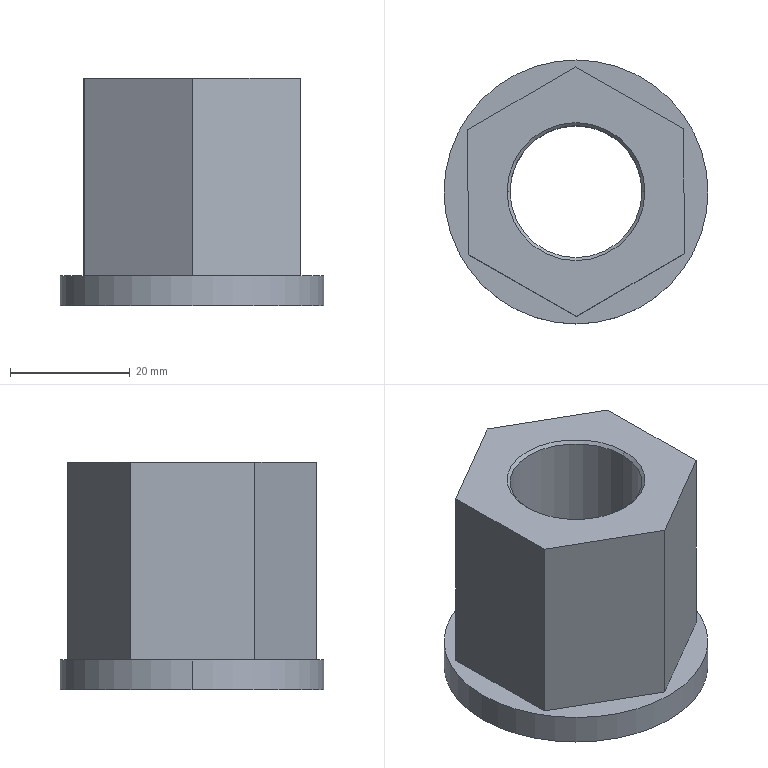Part | SolidWorks | features 3DProfileFeature 1, Boss 1, Chamfer 1, Extrusion 1, HoleWzd 1, RevCut 1 | 1 solid | 15 faces | box 44 x 44 x 38 mm | volume 30187 mm3 | plane 9 | cylinder 4 | cone 2 | commonest cylinder face diameters 22 x2 44 x2
STEP:
#1=CARTESIAN_POINT('',(-11.,0.,37.5));
#2=VERTEX_POINT('',#1);
#3=CARTESIAN_POINT('',(11.,0.,37.5));
#4=VERTEX_POINT('',#3);
#5=CARTESIAN_POINT('',(0.,0.,37.5));
#6=DIRECTION('',(0.,0.,1.));
#7=DIRECTION('',(-1.,0.,0.));
#8=AXIS2_PLACEMENT_3D('',#5,#6,#7);
#9=CIRCLE('',#8,11.);
#10=EDGE_CURVE('',#2,#4,#9,.T.);
#11=ORIENTED_EDGE('',*,*,#10,.F.);
#12=CARTESIAN_POINT('',(-11.5,0.,38.));
#13=VERTEX_POINT('',#12);
#14=CARTESIAN_POINT('',(-11.,0.,37.5));
#15=DIRECTION('',(-0.7071,0.,0.7071));
#16=VECTOR('',#15,1000.);
#17=LINE('',#14,#16);
#18=EDGE_CURVE('',#2,#13,#17,.T.);
#19=ORIENTED_EDGE('',*,*,#18,.T.);
#20=CARTESIAN_POINT('',(11.5,0.,38.));
#21=VERTEX_POINT('',#20);
#22=CARTESIAN_POINT('',(0.,0.,38.));
#23=DIRECTION('',(0.,0.,-1.));
#24=DIRECTION('',(-1.,0.,0.));
#25=AXIS2_PLACEMENT_3D('',#22,#23,#24);
#26=CIRCLE('',#25,11.5);
#27=EDGE_CURVE('',#21,#13,#26,.T.);
#28=ORIENTED_EDGE('',*,*,#27,.F.);
#29=CARTESIAN_POINT('',(11.,0.,37.5));
#30=DIRECTION('',(0.7071,0.,0.7071));
#31=VECTOR('',#30,1000.);
#32=LINE('',#29,#31);
#33=EDGE_CURVE('',#4,#21,#32,.T.);
#34=ORIENTED_EDGE('',*,*,#33,.F.);
#35=EDGE_LOOP('',(#11,#19,#28,#34));
#36=FACE_OUTER_BOUND('',#35,.T.);
#37=CARTESIAN_POINT('',(0.,0.,37.5));
#38=DIRECTION('',(0.,0.,1.));
#39=DIRECTION('',(1.,0.,0.));
#40=AXIS2_PLACEMENT_3D('',#37,#38,#39);
#41=CONICAL_SURFACE('',#40,11.,0.7854);
#42=ADVANCED_FACE('',(#36),#41,.F.);
#43=CARTESIAN_POINT('',(-11.,0.,0.));
#44=VERTEX_POINT('',#43);
#45=CARTESIAN_POINT('',(11.,0.,0.));
#46=VERTEX_POINT('',#45);
#47=CARTESIAN_POINT('',(0.,0.,0.));
#48=DIRECTION('',(0.,0.,1.));
#49=DIRECTION('',(1.,0.,0.));
#50=AXIS2_PLACEMENT_3D('',#47,#48,#49);
#51=CIRCLE('',#50,11.);
#52=EDGE_CURVE('',#44,#46,#51,.T.);
#53=ORIENTED_EDGE('',*,*,#52,.F.);
#54=CARTESIAN_POINT('',(-11.,0.,38.));
#55=DIRECTION('',(0.,0.,1.));
#56=VECTOR('',#55,1000.);
#57=LINE('',#54,#56);
#58=EDGE_CURVE('',#44,#2,#57,.T.);
#59=ORIENTED_EDGE('',*,*,#58,.T.);
#60=ORIENTED_EDGE('',*,*,#10,.T.);
#61=CARTESIAN_POINT('',(11.,0.,38.));
#62=DIRECTION('',(0.,0.,1.));
#63=VECTOR('',#62,1000.);
#64=LINE('',#61,#63);
#65=EDGE_CURVE('',#46,#4,#64,.T.);
#66=ORIENTED_EDGE('',*,*,#65,.F.);
#67=EDGE_LOOP('',(#53,#59,#60,#66));
#68=FACE_OUTER_BOUND('',#67,.T.);
#69=CARTESIAN_POINT('',(0.,0.,38.));
#70=DIRECTION('',(0.,0.,1.));
#71=DIRECTION('',(1.,0.,0.));
#72=AXIS2_PLACEMENT_3D('',#69,#70,#71);
#73=CYLINDRICAL_SURFACE('',#72,11.);
#74=ADVANCED_FACE('',(#68),#73,.F.);
#75=CARTESIAN_POINT('',(22.,0.,5.));
#76=VERTEX_POINT('',#75);
#77=CARTESIAN_POINT('',(-22.,0.,5.));
#78=VERTEX_POINT('',#77);
#79=CARTESIAN_POINT('',(0.,0.,5.));
#80=DIRECTION('',(0.,0.,1.));
#81=DIRECTION('',(1.,0.,0.));
#82=AXIS2_PLACEMENT_3D('',#79,#80,#81);
#83=CIRCLE('',#82,22.);
#84=EDGE_CURVE('',#76,#78,#83,.T.);
#85=ORIENTED_EDGE('',*,*,#84,.F.);
#86=CARTESIAN_POINT('',(22.,0.,0.));
#87=VERTEX_POINT('',#86);
#88=CARTESIAN_POINT('',(22.,0.,5.));
#89=DIRECTION('',(0.,0.,-1.));
#90=VECTOR('',#89,1000.);
#91=LINE('',#88,#90);
#92=EDGE_CURVE('',#76,#87,#91,.T.);
#93=ORIENTED_EDGE('',*,*,#92,.T.);
#94=CARTESIAN_POINT('',(-22.,0.,0.));
#95=VERTEX_POINT('',#94);
#96=CARTESIAN_POINT('',(0.,0.,0.));
#97=DIRECTION('',(0.,0.,1.));
#98=DIRECTION('',(1.,0.,0.));
#99=AXIS2_PLACEMENT_3D('',#96,#97,#98);
#100=CIRCLE('',#99,22.);
#101=EDGE_CURVE('',#87,#95,#100,.T.);
#102=ORIENTED_EDGE('',*,*,#101,.T.);
#103=CARTESIAN_POINT('',(-22.,0.,5.));
#104=DIRECTION('',(0.,0.,-1.));
#105=VECTOR('',#104,1000.);
#106=LINE('',#103,#105);
#107=EDGE_CURVE('',#78,#95,#106,.T.);
#108=ORIENTED_EDGE('',*,*,#107,.F.);
#109=EDGE_LOOP('',(#85,#93,#102,#108));
#110=FACE_OUTER_BOUND('',#109,.T.);
#111=CARTESIAN_POINT('',(0.,0.,5.));
#112=DIRECTION('',(0.,0.,-1.));
#113=DIRECTION('',(-1.,0.,0.));
#114=AXIS2_PLACEMENT_3D('',#111,#112,#113);
#115=CYLINDRICAL_SURFACE('',#114,22.);
#116=ADVANCED_FACE('',(#110),#115,.T.);
#117=CARTESIAN_POINT('',(0.,0.,5.));
#118=DIRECTION('',(0.,0.,1.));
#119=DIRECTION('',(1.,0.,0.));
#120=AXIS2_PLACEMENT_3D('',#117,#118,#119);
#121=CIRCLE('',#120,22.);
#122=EDGE_CURVE('',#78,#76,#121,.T.);
#123=ORIENTED_EDGE('',*,*,#122,.T.);
#124=ORIENTED_EDGE('',*,*,#84,.T.);
#125=EDGE_LOOP('',(#123,#124));
#126=FACE_OUTER_BOUND('',#125,.T.);
#127=CARTESIAN_POINT('',(-17.946,-10.485,5.));
#128=VERTEX_POINT('',#127);
#129=CARTESIAN_POINT('',(0.1075,-20.784,5.));
#130=VERTEX_POINT('',#129);
#131=CARTESIAN_POINT('',(-17.946,-10.485,5.));
#132=DIRECTION('',(0.8686,-0.4955,0.));
#133=VECTOR('',#132,1000.);
#134=LINE('',#131,#133);
#135=EDGE_CURVE('',#128,#130,#134,.T.);
#136=ORIENTED_EDGE('',*,*,#135,.F.);
#137=CARTESIAN_POINT('',(-18.054,10.299,5.));
#138=VERTEX_POINT('',#137);
#139=CARTESIAN_POINT('',(-18.054,10.299,5.));
#140=DIRECTION('',(0.005174,-1.,0.));
#141=VECTOR('',#140,1000.);
#142=LINE('',#139,#141);
#143=EDGE_CURVE('',#138,#128,#142,.T.);
#144=ORIENTED_EDGE('',*,*,#143,.F.);
#145=CARTESIAN_POINT('',(-0.1075,20.784,5.));
#146=VERTEX_POINT('',#145);
#147=CARTESIAN_POINT('',(-0.1075,20.784,5.));
#148=DIRECTION('',(-0.8634,-0.5045,0.));
#149=VECTOR('',#148,1000.);
#150=LINE('',#147,#149);
#151=EDGE_CURVE('',#146,#138,#150,.T.);
#152=ORIENTED_EDGE('',*,*,#151,.F.);
#153=CARTESIAN_POINT('',(17.946,10.485,5.));
#154=VERTEX_POINT('',#153);
#155=CARTESIAN_POINT('',(17.946,10.485,5.));
#156=DIRECTION('',(-0.8686,0.4955,0.));
#157=VECTOR('',#156,1000.);
#158=LINE('',#155,#157);
#159=EDGE_CURVE('',#154,#146,#158,.T.);
#160=ORIENTED_EDGE('',*,*,#159,.F.);
#161=CARTESIAN_POINT('',(18.054,-10.299,5.));
#162=VERTEX_POINT('',#161);
#163=CARTESIAN_POINT('',(18.054,-10.299,5.));
#164=DIRECTION('',(-0.005174,1.,0.));
#165=VECTOR('',#164,1000.);
#166=LINE('',#163,#165);
#167=EDGE_CURVE('',#162,#154,#166,.T.);
#168=ORIENTED_EDGE('',*,*,#167,.F.);
#169=CARTESIAN_POINT('',(0.1075,-20.784,5.));
#170=DIRECTION('',(0.8634,0.5045,0.));
#171=VECTOR('',#170,1000.);
#172=LINE('',#169,#171);
#173=EDGE_CURVE('',#130,#162,#172,.T.);
#174=ORIENTED_EDGE('',*,*,#173,.F.);
#175=EDGE_LOOP('',(#136,#144,#152,#160,#168,#174));
#176=FACE_BOUND('',#175,.T.);
#177=CARTESIAN_POINT('',(0.,0.,5.));
#178=DIRECTION('',(0.,0.,1.));
#179=DIRECTION('',(1.,0.,0.));
#180=AXIS2_PLACEMENT_3D('',#177,#178,#179);
#181=PLANE('',#180);
#182=ADVANCED_FACE('',(#126,#176),#181,.T.);
#183=ORIENTED_EDGE('',*,*,#92,.F.);
#184=ORIENTED_EDGE('',*,*,#122,.F.);
#185=ORIENTED_EDGE('',*,*,#107,.T.);
#186=CARTESIAN_POINT('',(0.,0.,0.));
#187=DIRECTION('',(0.,0.,1.));
#188=DIRECTION('',(1.,0.,0.));
#189=AXIS2_PLACEMENT_3D('',#186,#187,#188);
#190=CIRCLE('',#189,22.);
#191=EDGE_CURVE('',#95,#87,#190,.T.);
#192=ORIENTED_EDGE('',*,*,#191,.T.);
#193=EDGE_LOOP('',(#183,#184,#185,#192));
#194=FACE_OUTER_BOUND('',#193,.T.);
#195=CARTESIAN_POINT('',(0.,0.,5.));
#196=DIRECTION('',(0.,0.,-1.));
#197=DIRECTION('',(-1.,0.,0.));
#198=AXIS2_PLACEMENT_3D('',#195,#196,#197);
#199=CYLINDRICAL_SURFACE('',#198,22.);
#200=ADVANCED_FACE('',(#194),#199,.T.);
#201=CARTESIAN_POINT('',(0.,0.,0.));
#202=DIRECTION('',(0.,0.,1.));
#203=DIRECTION('',(1.,0.,0.));
#204=AXIS2_PLACEMENT_3D('',#201,#202,#203);
#205=CIRCLE('',#204,11.);
#206=EDGE_CURVE('',#46,#44,#205,.T.);
#207=ORIENTED_EDGE('',*,*,#206,.T.);
#208=ORIENTED_EDGE('',*,*,#52,.T.);
#209=EDGE_LOOP('',(#207,#208));
#210=FACE_BOUND('',#209,.T.);
#211=ORIENTED_EDGE('',*,*,#191,.F.);
#212=ORIENTED_EDGE('',*,*,#101,.F.);
#213=EDGE_LOOP('',(#211,#212));
#214=FACE_OUTER_BOUND('',#213,.T.);
#215=CARTESIAN_POINT('',(0.,0.,0.));
#216=DIRECTION('',(0.,0.,1.));
#217=DIRECTION('',(1.,0.,0.));
#218=AXIS2_PLACEMENT_3D('',#215,#216,#217);
#219=PLANE('',#218);
#220=ADVANCED_FACE('',(#210,#214),#219,.F.);
#221=ORIENTED_EDGE('',*,*,#143,.T.);
#222=CARTESIAN_POINT('',(-17.946,-10.485,38.));
#223=VERTEX_POINT('',#222);
#224=CARTESIAN_POINT('',(-17.946,-10.485,38.));
#225=DIRECTION('',(0.,0.,-1.));
#226=VECTOR('',#225,1000.);
#227=LINE('',#224,#226);
#228=EDGE_CURVE('',#223,#128,#227,.T.);
#229=ORIENTED_EDGE('',*,*,#228,.F.);
#230=CARTESIAN_POINT('',(-18.054,10.299,38.));
#231=VERTEX_POINT('',#230);
#232=CARTESIAN_POINT('',(-18.054,10.299,38.));
#233=DIRECTION('',(0.005174,-1.,0.));
#234=VECTOR('',#233,1000.);
#235=LINE('',#232,#234);
#236=EDGE_CURVE('',#231,#223,#235,.T.);
#237=ORIENTED_EDGE('',*,*,#236,.F.);
#238=CARTESIAN_POINT('',(-18.054,10.299,38.));
#239=DIRECTION('',(0.,0.,-1.));
#240=VECTOR('',#239,1000.);
#241=LINE('',#238,#240);
#242=EDGE_CURVE('',#231,#138,#241,.T.);
#243=ORIENTED_EDGE('',*,*,#242,.T.);
#244=EDGE_LOOP('',(#221,#229,#237,#243));
#245=FACE_OUTER_BOUND('',#244,.T.);
#246=CARTESIAN_POINT('',(-18.054,10.299,38.));
#247=DIRECTION('',(1.,0.005174,0.));
#248=DIRECTION('',(-0.005174,1.,0.));
#249=AXIS2_PLACEMENT_3D('',#246,#247,#248);
#250=PLANE('',#249);
#251=ADVANCED_FACE('',(#245),#250,.F.);
#252=ORIENTED_EDGE('',*,*,#135,.T.);
#253=CARTESIAN_POINT('',(0.1075,-20.784,38.));
#254=VERTEX_POINT('',#253);
#255=CARTESIAN_POINT('',(0.1075,-20.784,38.));
#256=DIRECTION('',(0.,0.,-1.));
#257=VECTOR('',#256,1000.);
#258=LINE('',#255,#257);
#259=EDGE_CURVE('',#254,#130,#258,.T.);
#260=ORIENTED_EDGE('',*,*,#259,.F.);
#261=CARTESIAN_POINT('',(-17.946,-10.485,38.));
#262=DIRECTION('',(0.8686,-0.4955,0.));
#263=VECTOR('',#262,1000.);
#264=LINE('',#261,#263);
#265=EDGE_CURVE('',#223,#254,#264,.T.);
#266=ORIENTED_EDGE('',*,*,#265,.F.);
#267=ORIENTED_EDGE('',*,*,#228,.T.);
#268=EDGE_LOOP('',(#252,#260,#266,#267));
#269=FACE_OUTER_BOUND('',#268,.T.);
#270=CARTESIAN_POINT('',(-17.946,-10.485,38.));
#271=DIRECTION('',(0.4955,0.8686,0.));
#272=DIRECTION('',(-0.8686,0.4955,0.));
#273=AXIS2_PLACEMENT_3D('',#270,#271,#272);
#274=PLANE('',#273);
#275=ADVANCED_FACE('',(#269),#274,.F.);
#276=ORIENTED_EDGE('',*,*,#173,.T.);
#277=CARTESIAN_POINT('',(18.054,-10.299,38.));
#278=VERTEX_POINT('',#277);
#279=CARTESIAN_POINT('',(18.054,-10.299,38.));
#280=DIRECTION('',(0.,0.,-1.));
#281=VECTOR('',#280,1000.);
#282=LINE('',#279,#281);
#283=EDGE_CURVE('',#278,#162,#282,.T.);
#284=ORIENTED_EDGE('',*,*,#283,.F.);
#285=CARTESIAN_POINT('',(0.1075,-20.784,38.));
#286=DIRECTION('',(0.8634,0.5045,0.));
#287=VECTOR('',#286,1000.);
#288=LINE('',#285,#287);
#289=EDGE_CURVE('',#254,#278,#288,.T.);
#290=ORIENTED_EDGE('',*,*,#289,.F.);
#291=ORIENTED_EDGE('',*,*,#259,.T.);
#292=EDGE_LOOP('',(#276,#284,#290,#291));
#293=FACE_OUTER_BOUND('',#292,.T.);
#294=CARTESIAN_POINT('',(0.1075,-20.784,38.));
#295=DIRECTION('',(-0.5045,0.8634,0.));
#296=DIRECTION('',(-0.8634,-0.5045,0.));
#297=AXIS2_PLACEMENT_3D('',#294,#295,#296);
#298=PLANE('',#297);
#299=ADVANCED_FACE('',(#293),#298,.F.);
#300=ORIENTED_EDGE('',*,*,#167,.T.);
#301=CARTESIAN_POINT('',(17.946,10.485,38.));
#302=VERTEX_POINT('',#301);
#303=CARTESIAN_POINT('',(17.946,10.485,38.));
#304=DIRECTION('',(0.,0.,-1.));
#305=VECTOR('',#304,1000.);
#306=LINE('',#303,#305);
#307=EDGE_CURVE('',#302,#154,#306,.T.);
#308=ORIENTED_EDGE('',*,*,#307,.F.);
#309=CARTESIAN_POINT('',(18.054,-10.299,38.));
#310=DIRECTION('',(-0.005174,1.,0.));
#311=VECTOR('',#310,1000.);
#312=LINE('',#309,#311);
#313=EDGE_CURVE('',#278,#302,#312,.T.);
#314=ORIENTED_EDGE('',*,*,#313,.F.);
#315=ORIENTED_EDGE('',*,*,#283,.T.);
#316=EDGE_LOOP('',(#300,#308,#314,#315));
#317=FACE_OUTER_BOUND('',#316,.T.);
#318=CARTESIAN_POINT('',(18.054,-10.299,38.));
#319=DIRECTION('',(-1.,-0.005174,0.));
#320=DIRECTION('',(0.005174,-1.,0.));
#321=AXIS2_PLACEMENT_3D('',#318,#319,#320);
#322=PLANE('',#321);
#323=ADVANCED_FACE('',(#317),#322,.F.);
#324=ORIENTED_EDGE('',*,*,#159,.T.);
#325=CARTESIAN_POINT('',(-0.1075,20.784,38.));
#326=VERTEX_POINT('',#325);
#327=CARTESIAN_POINT('',(-0.1075,20.784,38.));
#328=DIRECTION('',(0.,0.,-1.));
#329=VECTOR('',#328,1000.);
#330=LINE('',#327,#329);
#331=EDGE_CURVE('',#326,#146,#330,.T.);
#332=ORIENTED_EDGE('',*,*,#331,.F.);
#333=CARTESIAN_POINT('',(17.946,10.485,38.));
#334=DIRECTION('',(-0.8686,0.4955,0.));
#335=VECTOR('',#334,1000.);
#336=LINE('',#333,#335);
#337=EDGE_CURVE('',#302,#326,#336,.T.);
#338=ORIENTED_EDGE('',*,*,#337,.F.);
#339=ORIENTED_EDGE('',*,*,#307,.T.);
#340=EDGE_LOOP('',(#324,#332,#338,#339));
#341=FACE_OUTER_BOUND('',#340,.T.);
#342=CARTESIAN_POINT('',(17.946,10.485,38.));
#343=DIRECTION('',(-0.4955,-0.8686,0.));
#344=DIRECTION('',(0.8686,-0.4955,0.));
#345=AXIS2_PLACEMENT_3D('',#342,#343,#344);
#346=PLANE('',#345);
#347=ADVANCED_FACE('',(#341),#346,.F.);
#348=ORIENTED_EDGE('',*,*,#151,.T.);
#349=ORIENTED_EDGE('',*,*,#242,.F.);
#350=CARTESIAN_POINT('',(-0.1075,20.784,38.));
#351=DIRECTION('',(-0.8634,-0.5045,0.));
#352=VECTOR('',#351,1000.);
#353=LINE('',#350,#352);
#354=EDGE_CURVE('',#326,#231,#353,.T.);
#355=ORIENTED_EDGE('',*,*,#354,.F.);
#356=ORIENTED_EDGE('',*,*,#331,.T.);
#357=EDGE_LOOP('',(#348,#349,#355,#356));
#358=FACE_OUTER_BOUND('',#357,.T.);
#359=CARTESIAN_POINT('',(-0.1075,20.784,38.));
#360=DIRECTION('',(0.5045,-0.8634,0.));
#361=DIRECTION('',(0.8634,0.5045,0.));
#362=AXIS2_PLACEMENT_3D('',#359,#360,#361);
#363=PLANE('',#362);
#364=ADVANCED_FACE('',(#358),#363,.F.);
#365=ORIENTED_EDGE('',*,*,#27,.T.);
#366=CARTESIAN_POINT('',(0.,0.,38.));
#367=DIRECTION('',(0.,0.,-1.));
#368=DIRECTION('',(-1.,0.,0.));
#369=AXIS2_PLACEMENT_3D('',#366,#367,#368);
#370=CIRCLE('',#369,11.5);
#371=EDGE_CURVE('',#13,#21,#370,.T.);
#372=ORIENTED_EDGE('',*,*,#371,.T.);
#373=EDGE_LOOP('',(#365,#372));
#374=FACE_BOUND('',#373,.T.);
#375=ORIENTED_EDGE('',*,*,#236,.T.);
#376=ORIENTED_EDGE('',*,*,#265,.T.);
#377=ORIENTED_EDGE('',*,*,#289,.T.);
#378=ORIENTED_EDGE('',*,*,#313,.T.);
#379=ORIENTED_EDGE('',*,*,#337,.T.);
#380=ORIENTED_EDGE('',*,*,#354,.T.);
#381=EDGE_LOOP('',(#375,#376,#377,#378,#379,#380));
#382=FACE_OUTER_BOUND('',#381,.T.);
#383=CARTESIAN_POINT('',(-18.161,31.083,38.));
#384=DIRECTION('',(0.,0.,-1.));
#385=DIRECTION('',(-1.,0.,0.));
#386=AXIS2_PLACEMENT_3D('',#383,#384,#385);
#387=PLANE('',#386);
#388=ADVANCED_FACE('',(#374,#382),#387,.F.);
#389=ORIENTED_EDGE('',*,*,#58,.F.);
#390=ORIENTED_EDGE('',*,*,#206,.F.);
#391=ORIENTED_EDGE('',*,*,#65,.T.);
#392=CARTESIAN_POINT('',(0.,0.,37.5));
#393=DIRECTION('',(0.,0.,1.));
#394=DIRECTION('',(-1.,0.,0.));
#395=AXIS2_PLACEMENT_3D('',#392,#393,#394);
#396=CIRCLE('',#395,11.);
#397=EDGE_CURVE('',#4,#2,#396,.T.);
#398=ORIENTED_EDGE('',*,*,#397,.T.);
#399=EDGE_LOOP('',(#389,#390,#391,#398));
#400=FACE_OUTER_BOUND('',#399,.T.);
#401=CARTESIAN_POINT('',(0.,0.,38.));
#402=DIRECTION('',(0.,0.,1.));
#403=DIRECTION('',(1.,0.,0.));
#404=AXIS2_PLACEMENT_3D('',#401,#402,#403);
#405=CYLINDRICAL_SURFACE('',#404,11.);
#406=ADVANCED_FACE('',(#400),#405,.F.);
#407=ORIENTED_EDGE('',*,*,#18,.F.);
#408=ORIENTED_EDGE('',*,*,#397,.F.);
#409=ORIENTED_EDGE('',*,*,#33,.T.);
#410=ORIENTED_EDGE('',*,*,#371,.F.);
#411=EDGE_LOOP('',(#407,#408,#409,#410));
#412=FACE_OUTER_BOUND('',#411,.T.);
#413=CARTESIAN_POINT('',(0.,0.,37.5));
#414=DIRECTION('',(0.,0.,1.));
#415=DIRECTION('',(1.,0.,0.));
#416=AXIS2_PLACEMENT_3D('',#413,#414,#415);
#417=CONICAL_SURFACE('',#416,11.,0.7854);
#418=ADVANCED_FACE('',(#412),#417,.F.);
#419=CLOSED_SHELL('',(#42,#74,#116,#182,#200,#220,#251,#275,#299,#323,#347,#364,#388,#406,#418));
#420=MANIFOLD_SOLID_BREP('',#419);
#421=CARTESIAN_POINT('',(0.,0.,0.));
#422=DIRECTION('',(0.,0.,1.));
#423=DIRECTION('',(1.,0.,0.));
#424=AXIS2_PLACEMENT_3D('',#421,#422,#423);
#425=(LENGTH_UNIT()NAMED_UNIT(*)SI_UNIT(.MILLI.,.METRE.));
#426=UNCERTAINTY_MEASURE_WITH_UNIT(LENGTH_MEASURE(0.00001),#425,'','');
#427=(NAMED_UNIT(*)PLANE_ANGLE_UNIT()SI_UNIT($,.RADIAN.));
#428=(NAMED_UNIT(*)SI_UNIT($,.STERADIAN.)SOLID_ANGLE_UNIT());
#429=(GEOMETRIC_REPRESENTATION_CONTEXT(3)GLOBAL_UNCERTAINTY_ASSIGNED_CONTEXT((#426))GLOBAL_UNIT_ASSIGNED_CONTEXT((#425,#427,#428))REPRESENTATION_CONTEXT('',''));
#430=ADVANCED_BREP_SHAPE_REPRESENTATION('',(#420,#424),#429);